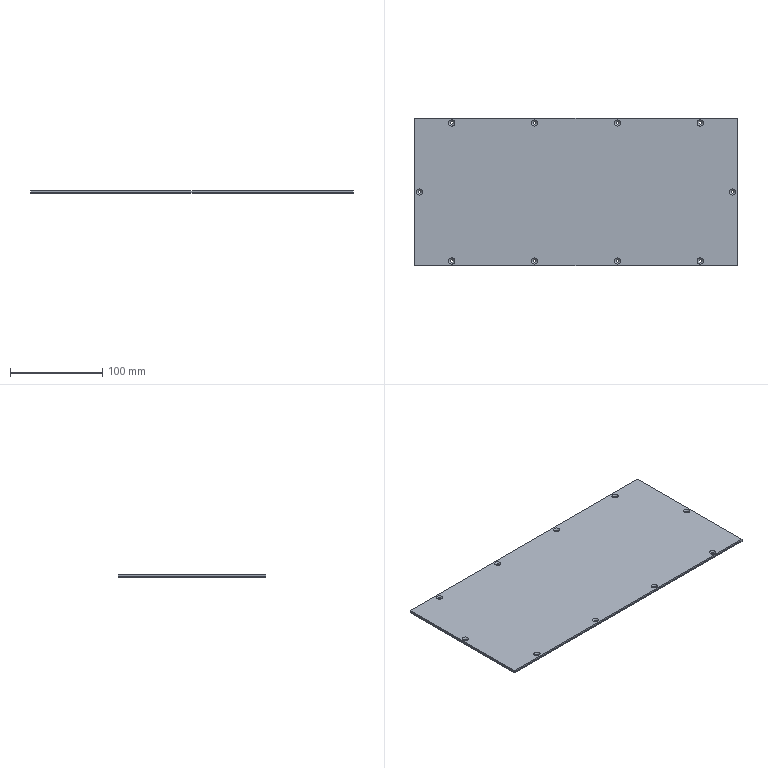Part | SolidWorks | features BaseBody 2 | 2 solids | 72 faces | box 350 x 160 x 3 mm | volume 167533 mm3 | cylinder 40 | cone 20 | plane 12 | commonest cylinder face diameters 3.4 x40